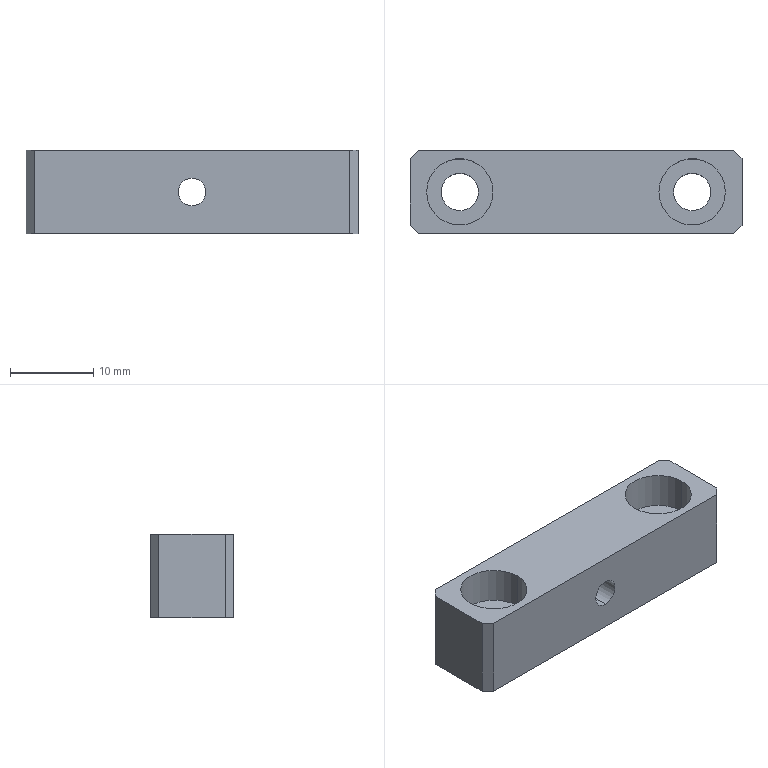Part | STEP file | 11-FG-B08511 | 1 solid | 22 faces | box 40 x 10 x 10 mm | volume 3274 mm3 | plane 12 | cylinder 10 | commonest cylinder face diameters 4.5 x4 8 x4 3.3 x2
STEP:
#1=CARTESIAN_POINT('',(0.,5.,6.65));
#2=VERTEX_POINT('',#1);
#3=CARTESIAN_POINT('',(0.,5.,3.35));
#4=VERTEX_POINT('',#3);
#5=CARTESIAN_POINT('',(0.,5.,5.));
#6=DIRECTION('',(0.,-1.,0.));
#7=DIRECTION('',(0.,0.,-1.));
#8=AXIS2_PLACEMENT_3D('',#5,#6,#7);
#9=CIRCLE('',#8,1.65);
#10=EDGE_CURVE('',#2,#4,#9,.T.);
#11=ORIENTED_EDGE('',*,*,#10,.F.);
#12=CARTESIAN_POINT('',(0.,-5.,6.65));
#13=VERTEX_POINT('',#12);
#14=CARTESIAN_POINT('',(0.,-5.,6.65));
#15=DIRECTION('',(0.,-1.,0.));
#16=VECTOR('',#15,1000.);
#17=LINE('',#14,#16);
#18=EDGE_CURVE('',#2,#13,#17,.T.);
#19=ORIENTED_EDGE('',*,*,#18,.T.);
#20=CARTESIAN_POINT('',(0.,-5.,3.35));
#21=VERTEX_POINT('',#20);
#22=CARTESIAN_POINT('',(0.,-5.,5.));
#23=DIRECTION('',(0.,-1.,0.));
#24=DIRECTION('',(0.,0.,-1.));
#25=AXIS2_PLACEMENT_3D('',#22,#23,#24);
#26=CIRCLE('',#25,1.65);
#27=EDGE_CURVE('',#13,#21,#26,.T.);
#28=ORIENTED_EDGE('',*,*,#27,.T.);
#29=CARTESIAN_POINT('',(0.,-5.,3.35));
#30=DIRECTION('',(0.,-1.,0.));
#31=VECTOR('',#30,1000.);
#32=LINE('',#29,#31);
#33=EDGE_CURVE('',#4,#21,#32,.T.);
#34=ORIENTED_EDGE('',*,*,#33,.F.);
#35=EDGE_LOOP('',(#11,#19,#28,#34));
#36=FACE_OUTER_BOUND('',#35,.T.);
#37=CARTESIAN_POINT('',(0.,-5.,5.));
#38=DIRECTION('',(0.,-1.,0.));
#39=DIRECTION('',(0.,0.,-1.));
#40=AXIS2_PLACEMENT_3D('',#37,#38,#39);
#41=CYLINDRICAL_SURFACE('',#40,1.65);
#42=ADVANCED_FACE('',(#36),#41,.F.);
#43=CARTESIAN_POINT('',(-18.,0.,5.6));
#44=VERTEX_POINT('',#43);
#45=CARTESIAN_POINT('',(-10.,0.,5.6));
#46=VERTEX_POINT('',#45);
#47=CARTESIAN_POINT('',(-14.,0.,5.6));
#48=DIRECTION('',(0.,0.,1.));
#49=DIRECTION('',(1.,0.,0.));
#50=AXIS2_PLACEMENT_3D('',#47,#48,#49);
#51=CIRCLE('',#50,4.);
#52=EDGE_CURVE('',#44,#46,#51,.T.);
#53=ORIENTED_EDGE('',*,*,#52,.F.);
#54=CARTESIAN_POINT('',(-18.,0.,10.));
#55=VERTEX_POINT('',#54);
#56=CARTESIAN_POINT('',(-18.,0.,10.));
#57=DIRECTION('',(0.,0.,1.));
#58=VECTOR('',#57,1000.);
#59=LINE('',#56,#58);
#60=EDGE_CURVE('',#44,#55,#59,.T.);
#61=ORIENTED_EDGE('',*,*,#60,.T.);
#62=CARTESIAN_POINT('',(-10.,0.,10.));
#63=VERTEX_POINT('',#62);
#64=CARTESIAN_POINT('',(-14.,0.,10.));
#65=DIRECTION('',(0.,0.,1.));
#66=DIRECTION('',(1.,0.,0.));
#67=AXIS2_PLACEMENT_3D('',#64,#65,#66);
#68=CIRCLE('',#67,4.);
#69=EDGE_CURVE('',#55,#63,#68,.T.);
#70=ORIENTED_EDGE('',*,*,#69,.T.);
#71=CARTESIAN_POINT('',(-10.,0.,10.));
#72=DIRECTION('',(0.,0.,1.));
#73=VECTOR('',#72,1000.);
#74=LINE('',#71,#73);
#75=EDGE_CURVE('',#46,#63,#74,.T.);
#76=ORIENTED_EDGE('',*,*,#75,.F.);
#77=EDGE_LOOP('',(#53,#61,#70,#76));
#78=FACE_OUTER_BOUND('',#77,.T.);
#79=CARTESIAN_POINT('',(-14.,0.,10.));
#80=DIRECTION('',(0.,0.,1.));
#81=DIRECTION('',(1.,0.,0.));
#82=AXIS2_PLACEMENT_3D('',#79,#80,#81);
#83=CYLINDRICAL_SURFACE('',#82,4.);
#84=ADVANCED_FACE('',(#78),#83,.F.);
#85=CARTESIAN_POINT('',(-11.75,0.,0.));
#86=VERTEX_POINT('',#85);
#87=CARTESIAN_POINT('',(-16.25,0.,0.));
#88=VERTEX_POINT('',#87);
#89=CARTESIAN_POINT('',(-14.,0.,0.));
#90=DIRECTION('',(0.,0.,-1.));
#91=DIRECTION('',(-1.,0.,0.));
#92=AXIS2_PLACEMENT_3D('',#89,#90,#91);
#93=CIRCLE('',#92,2.25);
#94=EDGE_CURVE('',#86,#88,#93,.T.);
#95=ORIENTED_EDGE('',*,*,#94,.T.);
#96=CARTESIAN_POINT('',(-16.25,0.,5.6));
#97=VERTEX_POINT('',#96);
#98=CARTESIAN_POINT('',(-16.25,0.,10.));
#99=DIRECTION('',(0.,0.,1.));
#100=VECTOR('',#99,1000.);
#101=LINE('',#98,#100);
#102=EDGE_CURVE('',#88,#97,#101,.T.);
#103=ORIENTED_EDGE('',*,*,#102,.T.);
#104=CARTESIAN_POINT('',(-11.75,0.,5.6));
#105=VERTEX_POINT('',#104);
#106=CARTESIAN_POINT('',(-14.,0.,5.6));
#107=DIRECTION('',(0.,0.,1.));
#108=DIRECTION('',(1.,0.,0.));
#109=AXIS2_PLACEMENT_3D('',#106,#107,#108);
#110=CIRCLE('',#109,2.25);
#111=EDGE_CURVE('',#97,#105,#110,.T.);
#112=ORIENTED_EDGE('',*,*,#111,.T.);
#113=CARTESIAN_POINT('',(-11.75,0.,10.));
#114=DIRECTION('',(0.,0.,1.));
#115=VECTOR('',#114,1000.);
#116=LINE('',#113,#115);
#117=EDGE_CURVE('',#86,#105,#116,.T.);
#118=ORIENTED_EDGE('',*,*,#117,.F.);
#119=EDGE_LOOP('',(#95,#103,#112,#118));
#120=FACE_OUTER_BOUND('',#119,.T.);
#121=CARTESIAN_POINT('',(-14.,0.,10.));
#122=DIRECTION('',(0.,0.,1.));
#123=DIRECTION('',(1.,0.,0.));
#124=AXIS2_PLACEMENT_3D('',#121,#122,#123);
#125=CYLINDRICAL_SURFACE('',#124,2.25);
#126=ADVANCED_FACE('',(#120),#125,.F.);
#127=CARTESIAN_POINT('',(10.,0.,5.6));
#128=VERTEX_POINT('',#127);
#129=CARTESIAN_POINT('',(18.,0.,5.6));
#130=VERTEX_POINT('',#129);
#131=CARTESIAN_POINT('',(14.,0.,5.6));
#132=DIRECTION('',(0.,0.,1.));
#133=DIRECTION('',(1.,0.,0.));
#134=AXIS2_PLACEMENT_3D('',#131,#132,#133);
#135=CIRCLE('',#134,4.);
#136=EDGE_CURVE('',#128,#130,#135,.T.);
#137=ORIENTED_EDGE('',*,*,#136,.F.);
#138=CARTESIAN_POINT('',(10.,0.,10.));
#139=VERTEX_POINT('',#138);
#140=CARTESIAN_POINT('',(10.,0.,10.));
#141=DIRECTION('',(0.,0.,1.));
#142=VECTOR('',#141,1000.);
#143=LINE('',#140,#142);
#144=EDGE_CURVE('',#128,#139,#143,.T.);
#145=ORIENTED_EDGE('',*,*,#144,.T.);
#146=CARTESIAN_POINT('',(18.,0.,10.));
#147=VERTEX_POINT('',#146);
#148=CARTESIAN_POINT('',(14.,0.,10.));
#149=DIRECTION('',(0.,0.,1.));
#150=DIRECTION('',(1.,0.,0.));
#151=AXIS2_PLACEMENT_3D('',#148,#149,#150);
#152=CIRCLE('',#151,4.);
#153=EDGE_CURVE('',#139,#147,#152,.T.);
#154=ORIENTED_EDGE('',*,*,#153,.T.);
#155=CARTESIAN_POINT('',(18.,0.,10.));
#156=DIRECTION('',(0.,0.,1.));
#157=VECTOR('',#156,1000.);
#158=LINE('',#155,#157);
#159=EDGE_CURVE('',#130,#147,#158,.T.);
#160=ORIENTED_EDGE('',*,*,#159,.F.);
#161=EDGE_LOOP('',(#137,#145,#154,#160));
#162=FACE_OUTER_BOUND('',#161,.T.);
#163=CARTESIAN_POINT('',(14.,0.,10.));
#164=DIRECTION('',(0.,0.,1.));
#165=DIRECTION('',(1.,0.,0.));
#166=AXIS2_PLACEMENT_3D('',#163,#164,#165);
#167=CYLINDRICAL_SURFACE('',#166,4.);
#168=ADVANCED_FACE('',(#162),#167,.F.);
#169=CARTESIAN_POINT('',(16.25,0.,0.));
#170=VERTEX_POINT('',#169);
#171=CARTESIAN_POINT('',(11.75,0.,0.));
#172=VERTEX_POINT('',#171);
#173=CARTESIAN_POINT('',(14.,0.,0.));
#174=DIRECTION('',(0.,0.,-1.));
#175=DIRECTION('',(-1.,0.,0.));
#176=AXIS2_PLACEMENT_3D('',#173,#174,#175);
#177=CIRCLE('',#176,2.25);
#178=EDGE_CURVE('',#170,#172,#177,.T.);
#179=ORIENTED_EDGE('',*,*,#178,.T.);
#180=CARTESIAN_POINT('',(11.75,0.,5.6));
#181=VERTEX_POINT('',#180);
#182=CARTESIAN_POINT('',(11.75,0.,10.));
#183=DIRECTION('',(0.,0.,1.));
#184=VECTOR('',#183,1000.);
#185=LINE('',#182,#184);
#186=EDGE_CURVE('',#172,#181,#185,.T.);
#187=ORIENTED_EDGE('',*,*,#186,.T.);
#188=CARTESIAN_POINT('',(16.25,0.,5.6));
#189=VERTEX_POINT('',#188);
#190=CARTESIAN_POINT('',(14.,0.,5.6));
#191=DIRECTION('',(0.,0.,1.));
#192=DIRECTION('',(1.,0.,0.));
#193=AXIS2_PLACEMENT_3D('',#190,#191,#192);
#194=CIRCLE('',#193,2.25);
#195=EDGE_CURVE('',#181,#189,#194,.T.);
#196=ORIENTED_EDGE('',*,*,#195,.T.);
#197=CARTESIAN_POINT('',(16.25,0.,10.));
#198=DIRECTION('',(0.,0.,1.));
#199=VECTOR('',#198,1000.);
#200=LINE('',#197,#199);
#201=EDGE_CURVE('',#170,#189,#200,.T.);
#202=ORIENTED_EDGE('',*,*,#201,.F.);
#203=EDGE_LOOP('',(#179,#187,#196,#202));
#204=FACE_OUTER_BOUND('',#203,.T.);
#205=CARTESIAN_POINT('',(14.,0.,10.));
#206=DIRECTION('',(0.,0.,1.));
#207=DIRECTION('',(1.,0.,0.));
#208=AXIS2_PLACEMENT_3D('',#205,#206,#207);
#209=CYLINDRICAL_SURFACE('',#208,2.25);
#210=ADVANCED_FACE('',(#204),#209,.F.);
#211=CARTESIAN_POINT('',(20.,-4.,0.));
#212=VERTEX_POINT('',#211);
#213=CARTESIAN_POINT('',(20.,4.,0.));
#214=VERTEX_POINT('',#213);
#215=CARTESIAN_POINT('',(20.,-5.,0.));
#216=DIRECTION('',(0.,1.,0.));
#217=VECTOR('',#216,1000.);
#218=LINE('',#215,#217);
#219=EDGE_CURVE('',#212,#214,#218,.T.);
#220=ORIENTED_EDGE('',*,*,#219,.T.);
#221=CARTESIAN_POINT('',(20.,4.,10.));
#222=VERTEX_POINT('',#221);
#223=CARTESIAN_POINT('',(20.,4.,10.));
#224=DIRECTION('',(0.,0.,1.));
#225=VECTOR('',#224,1000.);
#226=LINE('',#223,#225);
#227=EDGE_CURVE('',#214,#222,#226,.T.);
#228=ORIENTED_EDGE('',*,*,#227,.T.);
#229=CARTESIAN_POINT('',(20.,-4.,10.));
#230=VERTEX_POINT('',#229);
#231=CARTESIAN_POINT('',(20.,-5.,10.));
#232=DIRECTION('',(0.,1.,0.));
#233=VECTOR('',#232,1000.);
#234=LINE('',#231,#233);
#235=EDGE_CURVE('',#230,#222,#234,.T.);
#236=ORIENTED_EDGE('',*,*,#235,.F.);
#237=CARTESIAN_POINT('',(20.,-4.,10.));
#238=DIRECTION('',(0.,0.,-1.));
#239=VECTOR('',#238,1000.);
#240=LINE('',#237,#239);
#241=EDGE_CURVE('',#230,#212,#240,.T.);
#242=ORIENTED_EDGE('',*,*,#241,.T.);
#243=EDGE_LOOP('',(#220,#228,#236,#242));
#244=FACE_OUTER_BOUND('',#243,.T.);
#245=CARTESIAN_POINT('',(20.,-5.,10.));
#246=DIRECTION('',(-1.,0.,0.));
#247=DIRECTION('',(0.,0.,1.));
#248=AXIS2_PLACEMENT_3D('',#245,#246,#247);
#249=PLANE('',#248);
#250=ADVANCED_FACE('',(#244),#249,.F.);
#251=CARTESIAN_POINT('',(0.,5.,5.));
#252=DIRECTION('',(0.,-1.,0.));
#253=DIRECTION('',(0.,0.,-1.));
#254=AXIS2_PLACEMENT_3D('',#251,#252,#253);
#255=CIRCLE('',#254,1.65);
#256=EDGE_CURVE('',#4,#2,#255,.T.);
#257=ORIENTED_EDGE('',*,*,#256,.T.);
#258=ORIENTED_EDGE('',*,*,#10,.T.);
#259=EDGE_LOOP('',(#257,#258));
#260=FACE_BOUND('',#259,.T.);
#261=CARTESIAN_POINT('',(19.,5.,10.));
#262=VERTEX_POINT('',#261);
#263=CARTESIAN_POINT('',(-19.,5.,10.));
#264=VERTEX_POINT('',#263);
#265=CARTESIAN_POINT('',(-20.,5.,10.));
#266=DIRECTION('',(-1.,0.,0.));
#267=VECTOR('',#266,1000.);
#268=LINE('',#265,#267);
#269=EDGE_CURVE('',#262,#264,#268,.T.);
#270=ORIENTED_EDGE('',*,*,#269,.F.);
#271=CARTESIAN_POINT('',(19.,5.,0.));
#272=VERTEX_POINT('',#271);
#273=CARTESIAN_POINT('',(19.,5.,10.));
#274=DIRECTION('',(0.,0.,-1.));
#275=VECTOR('',#274,1000.);
#276=LINE('',#273,#275);
#277=EDGE_CURVE('',#262,#272,#276,.T.);
#278=ORIENTED_EDGE('',*,*,#277,.T.);
#279=CARTESIAN_POINT('',(-19.,5.,0.));
#280=VERTEX_POINT('',#279);
#281=CARTESIAN_POINT('',(-20.,5.,0.));
#282=DIRECTION('',(-1.,0.,0.));
#283=VECTOR('',#282,1000.);
#284=LINE('',#281,#283);
#285=EDGE_CURVE('',#272,#280,#284,.T.);
#286=ORIENTED_EDGE('',*,*,#285,.T.);
#287=CARTESIAN_POINT('',(-19.,5.,10.));
#288=DIRECTION('',(0.,0.,1.));
#289=VECTOR('',#288,1000.);
#290=LINE('',#287,#289);
#291=EDGE_CURVE('',#280,#264,#290,.T.);
#292=ORIENTED_EDGE('',*,*,#291,.T.);
#293=EDGE_LOOP('',(#270,#278,#286,#292));
#294=FACE_OUTER_BOUND('',#293,.T.);
#295=CARTESIAN_POINT('',(-20.,5.,10.));
#296=DIRECTION('',(0.,-1.,0.));
#297=DIRECTION('',(0.,0.,-1.));
#298=AXIS2_PLACEMENT_3D('',#295,#296,#297);
#299=PLANE('',#298);
#300=ADVANCED_FACE('',(#260,#294),#299,.F.);
#301=CARTESIAN_POINT('',(-20.,4.,0.));
#302=VERTEX_POINT('',#301);
#303=CARTESIAN_POINT('',(-20.,-4.,0.));
#304=VERTEX_POINT('',#303);
#305=CARTESIAN_POINT('',(-20.,-5.,0.));
#306=DIRECTION('',(0.,-1.,0.));
#307=VECTOR('',#306,1000.);
#308=LINE('',#305,#307);
#309=EDGE_CURVE('',#302,#304,#308,.T.);
#310=ORIENTED_EDGE('',*,*,#309,.T.);
#311=CARTESIAN_POINT('',(-20.,-4.,10.));
#312=VERTEX_POINT('',#311);
#313=CARTESIAN_POINT('',(-20.,-4.,10.));
#314=DIRECTION('',(0.,0.,1.));
#315=VECTOR('',#314,1000.);
#316=LINE('',#313,#315);
#317=EDGE_CURVE('',#304,#312,#316,.T.);
#318=ORIENTED_EDGE('',*,*,#317,.T.);
#319=CARTESIAN_POINT('',(-20.,4.,10.));
#320=VERTEX_POINT('',#319);
#321=CARTESIAN_POINT('',(-20.,-5.,10.));
#322=DIRECTION('',(0.,-1.,0.));
#323=VECTOR('',#322,1000.);
#324=LINE('',#321,#323);
#325=EDGE_CURVE('',#320,#312,#324,.T.);
#326=ORIENTED_EDGE('',*,*,#325,.F.);
#327=CARTESIAN_POINT('',(-20.,4.,10.));
#328=DIRECTION('',(0.,0.,-1.));
#329=VECTOR('',#328,1000.);
#330=LINE('',#327,#329);
#331=EDGE_CURVE('',#320,#302,#330,.T.);
#332=ORIENTED_EDGE('',*,*,#331,.T.);
#333=EDGE_LOOP('',(#310,#318,#326,#332));
#334=FACE_OUTER_BOUND('',#333,.T.);
#335=CARTESIAN_POINT('',(-20.,-5.,10.));
#336=DIRECTION('',(1.,0.,0.));
#337=DIRECTION('',(0.,0.,-1.));
#338=AXIS2_PLACEMENT_3D('',#335,#336,#337);
#339=PLANE('',#338);
#340=ADVANCED_FACE('',(#334),#339,.F.);
#341=CARTESIAN_POINT('',(0.,-5.,5.));
#342=DIRECTION('',(0.,-1.,0.));
#343=DIRECTION('',(0.,0.,-1.));
#344=AXIS2_PLACEMENT_3D('',#341,#342,#343);
#345=CIRCLE('',#344,1.65);
#346=EDGE_CURVE('',#21,#13,#345,.T.);
#347=ORIENTED_EDGE('',*,*,#346,.F.);
#348=ORIENTED_EDGE('',*,*,#27,.F.);
#349=EDGE_LOOP('',(#347,#348));
#350=FACE_BOUND('',#349,.T.);
#351=CARTESIAN_POINT('',(-19.,-5.,0.));
#352=VERTEX_POINT('',#351);
#353=CARTESIAN_POINT('',(19.,-5.,0.));
#354=VERTEX_POINT('',#353);
#355=CARTESIAN_POINT('',(-20.,-5.,0.));
#356=DIRECTION('',(1.,0.,0.));
#357=VECTOR('',#356,1000.);
#358=LINE('',#355,#357);
#359=EDGE_CURVE('',#352,#354,#358,.T.);
#360=ORIENTED_EDGE('',*,*,#359,.T.);
#361=CARTESIAN_POINT('',(19.,-5.,10.));
#362=VERTEX_POINT('',#361);
#363=CARTESIAN_POINT('',(19.,-5.,10.));
#364=DIRECTION('',(0.,0.,1.));
#365=VECTOR('',#364,1000.);
#366=LINE('',#363,#365);
#367=EDGE_CURVE('',#354,#362,#366,.T.);
#368=ORIENTED_EDGE('',*,*,#367,.T.);
#369=CARTESIAN_POINT('',(-19.,-5.,10.));
#370=VERTEX_POINT('',#369);
#371=CARTESIAN_POINT('',(-20.,-5.,10.));
#372=DIRECTION('',(1.,0.,0.));
#373=VECTOR('',#372,1000.);
#374=LINE('',#371,#373);
#375=EDGE_CURVE('',#370,#362,#374,.T.);
#376=ORIENTED_EDGE('',*,*,#375,.F.);
#377=CARTESIAN_POINT('',(-19.,-5.,10.));
#378=DIRECTION('',(0.,0.,-1.));
#379=VECTOR('',#378,1000.);
#380=LINE('',#377,#379);
#381=EDGE_CURVE('',#370,#352,#380,.T.);
#382=ORIENTED_EDGE('',*,*,#381,.T.);
#383=EDGE_LOOP('',(#360,#368,#376,#382));
#384=FACE_OUTER_BOUND('',#383,.T.);
#385=CARTESIAN_POINT('',(-20.,-5.,10.));
#386=DIRECTION('',(0.,1.,0.));
#387=DIRECTION('',(0.,0.,1.));
#388=AXIS2_PLACEMENT_3D('',#385,#386,#387);
#389=PLANE('',#388);
#390=ADVANCED_FACE('',(#350,#384),#389,.F.);
#391=CARTESIAN_POINT('',(-14.,0.,10.));
#392=DIRECTION('',(0.,0.,1.));
#393=DIRECTION('',(1.,0.,0.));
#394=AXIS2_PLACEMENT_3D('',#391,#392,#393);
#395=CIRCLE('',#394,4.);
#396=EDGE_CURVE('',#63,#55,#395,.T.);
#397=ORIENTED_EDGE('',*,*,#396,.F.);
#398=ORIENTED_EDGE('',*,*,#69,.F.);
#399=EDGE_LOOP('',(#397,#398));
#400=FACE_BOUND('',#399,.T.);
#401=CARTESIAN_POINT('',(14.,0.,10.));
#402=DIRECTION('',(0.,0.,1.));
#403=DIRECTION('',(1.,0.,0.));
#404=AXIS2_PLACEMENT_3D('',#401,#402,#403);
#405=CIRCLE('',#404,4.);
#406=EDGE_CURVE('',#147,#139,#405,.T.);
#407=ORIENTED_EDGE('',*,*,#406,.F.);
#408=ORIENTED_EDGE('',*,*,#153,.F.);
#409=EDGE_LOOP('',(#407,#408));
#410=FACE_BOUND('',#409,.T.);
#411=ORIENTED_EDGE('',*,*,#235,.T.);
#412=CARTESIAN_POINT('',(19.,5.,10.));
#413=DIRECTION('',(-0.7071,0.7071,0.));
#414=VECTOR('',#413,1000.);
#415=LINE('',#412,#414);
#416=EDGE_CURVE('',#222,#262,#415,.T.);
#417=ORIENTED_EDGE('',*,*,#416,.T.);
#418=ORIENTED_EDGE('',*,*,#269,.T.);
#419=CARTESIAN_POINT('',(-20.,4.,10.));
#420=DIRECTION('',(-0.7071,-0.7071,0.));
#421=VECTOR('',#420,1000.);
#422=LINE('',#419,#421);
#423=EDGE_CURVE('',#264,#320,#422,.T.);
#424=ORIENTED_EDGE('',*,*,#423,.T.);
#425=ORIENTED_EDGE('',*,*,#325,.T.);
#426=CARTESIAN_POINT('',(-19.,-5.,10.));
#427=DIRECTION('',(0.7071,-0.7071,0.));
#428=VECTOR('',#427,1000.);
#429=LINE('',#426,#428);
#430=EDGE_CURVE('',#312,#370,#429,.T.);
#431=ORIENTED_EDGE('',*,*,#430,.T.);
#432=ORIENTED_EDGE('',*,*,#375,.T.);
#433=CARTESIAN_POINT('',(20.,-4.,10.));
#434=DIRECTION('',(0.7071,0.7071,0.));
#435=VECTOR('',#434,1000.);
#436=LINE('',#433,#435);
#437=EDGE_CURVE('',#362,#230,#436,.T.);
#438=ORIENTED_EDGE('',*,*,#437,.T.);
#439=EDGE_LOOP('',(#411,#417,#418,#424,#425,#431,#432,#438));
#440=FACE_OUTER_BOUND('',#439,.T.);
#441=CARTESIAN_POINT('',(20.,5.,10.));
#442=DIRECTION('',(0.,0.,-1.));
#443=DIRECTION('',(-1.,0.,0.));
#444=AXIS2_PLACEMENT_3D('',#441,#442,#443);
#445=PLANE('',#444);
#446=ADVANCED_FACE('',(#400,#410,#440),#445,.F.);
#447=ORIENTED_EDGE('',*,*,#94,.F.);
#448=CARTESIAN_POINT('',(-14.,0.,0.));
#449=DIRECTION('',(0.,0.,-1.));
#450=DIRECTION('',(-1.,0.,0.));
#451=AXIS2_PLACEMENT_3D('',#448,#449,#450);
#452=CIRCLE('',#451,2.25);
#453=EDGE_CURVE('',#88,#86,#452,.T.);
#454=ORIENTED_EDGE('',*,*,#453,.F.);
#455=EDGE_LOOP('',(#447,#454));
#456=FACE_BOUND('',#455,.T.);
#457=ORIENTED_EDGE('',*,*,#178,.F.);
#458=CARTESIAN_POINT('',(14.,0.,0.));
#459=DIRECTION('',(0.,0.,-1.));
#460=DIRECTION('',(-1.,0.,0.));
#461=AXIS2_PLACEMENT_3D('',#458,#459,#460);
#462=CIRCLE('',#461,2.25);
#463=EDGE_CURVE('',#172,#170,#462,.T.);
#464=ORIENTED_EDGE('',*,*,#463,.F.);
#465=EDGE_LOOP('',(#457,#464));
#466=FACE_BOUND('',#465,.T.);
#467=ORIENTED_EDGE('',*,*,#285,.F.);
#468=CARTESIAN_POINT('',(19.5,4.5,0.));
#469=DIRECTION('',(0.7071,-0.7071,0.));
#470=VECTOR('',#469,1000.);
#471=LINE('',#468,#470);
#472=EDGE_CURVE('',#272,#214,#471,.T.);
#473=ORIENTED_EDGE('',*,*,#472,.T.);
#474=ORIENTED_EDGE('',*,*,#219,.F.);
#475=CARTESIAN_POINT('',(24.5,0.5,0.));
#476=DIRECTION('',(-0.7071,-0.7071,0.));
#477=VECTOR('',#476,1000.);
#478=LINE('',#475,#477);
#479=EDGE_CURVE('',#212,#354,#478,.T.);
#480=ORIENTED_EDGE('',*,*,#479,.T.);
#481=ORIENTED_EDGE('',*,*,#359,.F.);
#482=CARTESIAN_POINT('',(-4.5,-19.5,0.));
#483=DIRECTION('',(-0.7071,0.7071,0.));
#484=VECTOR('',#483,1000.);
#485=LINE('',#482,#484);
#486=EDGE_CURVE('',#352,#304,#485,.T.);
#487=ORIENTED_EDGE('',*,*,#486,.T.);
#488=ORIENTED_EDGE('',*,*,#309,.F.);
#489=CARTESIAN_POINT('',(0.5,24.5,0.));
#490=DIRECTION('',(0.7071,0.7071,0.));
#491=VECTOR('',#490,1000.);
#492=LINE('',#489,#491);
#493=EDGE_CURVE('',#302,#280,#492,.T.);
#494=ORIENTED_EDGE('',*,*,#493,.T.);
#495=EDGE_LOOP('',(#467,#473,#474,#480,#481,#487,#488,#494));
#496=FACE_OUTER_BOUND('',#495,.T.);
#497=CARTESIAN_POINT('',(20.,5.,0.));
#498=DIRECTION('',(0.,0.,-1.));
#499=DIRECTION('',(-1.,0.,0.));
#500=AXIS2_PLACEMENT_3D('',#497,#498,#499);
#501=PLANE('',#500);
#502=ADVANCED_FACE('',(#456,#466,#496),#501,.T.);
#503=ORIENTED_EDGE('',*,*,#416,.F.);
#504=ORIENTED_EDGE('',*,*,#227,.F.);
#505=ORIENTED_EDGE('',*,*,#472,.F.);
#506=ORIENTED_EDGE('',*,*,#277,.F.);
#507=EDGE_LOOP('',(#503,#504,#505,#506));
#508=FACE_OUTER_BOUND('',#507,.T.);
#509=CARTESIAN_POINT('',(19.,5.,10.));
#510=DIRECTION('',(-0.7071,-0.7071,0.));
#511=DIRECTION('',(0.,0.,-1.));
#512=AXIS2_PLACEMENT_3D('',#509,#510,#511);
#513=PLANE('',#512);
#514=ADVANCED_FACE('',(#508),#513,.F.);
#515=ORIENTED_EDGE('',*,*,#437,.F.);
#516=ORIENTED_EDGE('',*,*,#367,.F.);
#517=ORIENTED_EDGE('',*,*,#479,.F.);
#518=ORIENTED_EDGE('',*,*,#241,.F.);
#519=EDGE_LOOP('',(#515,#516,#517,#518));
#520=FACE_OUTER_BOUND('',#519,.T.);
#521=CARTESIAN_POINT('',(20.,-4.,10.));
#522=DIRECTION('',(-0.7071,0.7071,0.));
#523=DIRECTION('',(0.,0.,-1.));
#524=AXIS2_PLACEMENT_3D('',#521,#522,#523);
#525=PLANE('',#524);
#526=ADVANCED_FACE('',(#520),#525,.F.);
#527=ORIENTED_EDGE('',*,*,#430,.F.);
#528=ORIENTED_EDGE('',*,*,#317,.F.);
#529=ORIENTED_EDGE('',*,*,#486,.F.);
#530=ORIENTED_EDGE('',*,*,#381,.F.);
#531=EDGE_LOOP('',(#527,#528,#529,#530));
#532=FACE_OUTER_BOUND('',#531,.T.);
#533=CARTESIAN_POINT('',(-19.,-5.,10.));
#534=DIRECTION('',(0.7071,0.7071,0.));
#535=DIRECTION('',(0.,0.,-1.));
#536=AXIS2_PLACEMENT_3D('',#533,#534,#535);
#537=PLANE('',#536);
#538=ADVANCED_FACE('',(#532),#537,.F.);
#539=ORIENTED_EDGE('',*,*,#423,.F.);
#540=ORIENTED_EDGE('',*,*,#291,.F.);
#541=ORIENTED_EDGE('',*,*,#493,.F.);
#542=ORIENTED_EDGE('',*,*,#331,.F.);
#543=EDGE_LOOP('',(#539,#540,#541,#542));
#544=FACE_OUTER_BOUND('',#543,.T.);
#545=CARTESIAN_POINT('',(-20.,4.,10.));
#546=DIRECTION('',(0.7071,-0.7071,0.));
#547=DIRECTION('',(0.,0.,-1.));
#548=AXIS2_PLACEMENT_3D('',#545,#546,#547);
#549=PLANE('',#548);
#550=ADVANCED_FACE('',(#544),#549,.F.);
#551=ORIENTED_EDGE('',*,*,#186,.F.);
#552=ORIENTED_EDGE('',*,*,#463,.T.);
#553=ORIENTED_EDGE('',*,*,#201,.T.);
#554=CARTESIAN_POINT('',(14.,0.,5.6));
#555=DIRECTION('',(0.,0.,1.));
#556=DIRECTION('',(1.,0.,0.));
#557=AXIS2_PLACEMENT_3D('',#554,#555,#556);
#558=CIRCLE('',#557,2.25);
#559=EDGE_CURVE('',#189,#181,#558,.T.);
#560=ORIENTED_EDGE('',*,*,#559,.T.);
#561=EDGE_LOOP('',(#551,#552,#553,#560));
#562=FACE_OUTER_BOUND('',#561,.T.);
#563=CARTESIAN_POINT('',(14.,0.,10.));
#564=DIRECTION('',(0.,0.,1.));
#565=DIRECTION('',(1.,0.,0.));
#566=AXIS2_PLACEMENT_3D('',#563,#564,#565);
#567=CYLINDRICAL_SURFACE('',#566,2.25);
#568=ADVANCED_FACE('',(#562),#567,.F.);
#569=ORIENTED_EDGE('',*,*,#559,.F.);
#570=ORIENTED_EDGE('',*,*,#195,.F.);
#571=EDGE_LOOP('',(#569,#570));
#572=FACE_BOUND('',#571,.T.);
#573=CARTESIAN_POINT('',(14.,0.,5.6));
#574=DIRECTION('',(0.,0.,1.));
#575=DIRECTION('',(1.,0.,0.));
#576=AXIS2_PLACEMENT_3D('',#573,#574,#575);
#577=CIRCLE('',#576,4.);
#578=EDGE_CURVE('',#130,#128,#577,.T.);
#579=ORIENTED_EDGE('',*,*,#578,.T.);
#580=ORIENTED_EDGE('',*,*,#136,.T.);
#581=EDGE_LOOP('',(#579,#580));
#582=FACE_OUTER_BOUND('',#581,.T.);
#583=CARTESIAN_POINT('',(16.25,0.,5.6));
#584=DIRECTION('',(0.,0.,-1.));
#585=DIRECTION('',(-1.,0.,0.));
#586=AXIS2_PLACEMENT_3D('',#583,#584,#585);
#587=PLANE('',#586);
#588=ADVANCED_FACE('',(#572,#582),#587,.F.);
#589=ORIENTED_EDGE('',*,*,#144,.F.);
#590=ORIENTED_EDGE('',*,*,#578,.F.);
#591=ORIENTED_EDGE('',*,*,#159,.T.);
#592=ORIENTED_EDGE('',*,*,#406,.T.);
#593=EDGE_LOOP('',(#589,#590,#591,#592));
#594=FACE_OUTER_BOUND('',#593,.T.);
#595=CARTESIAN_POINT('',(14.,0.,10.));
#596=DIRECTION('',(0.,0.,1.));
#597=DIRECTION('',(1.,0.,0.));
#598=AXIS2_PLACEMENT_3D('',#595,#596,#597);
#599=CYLINDRICAL_SURFACE('',#598,4.);
#600=ADVANCED_FACE('',(#594),#599,.F.);
#601=ORIENTED_EDGE('',*,*,#102,.F.);
#602=ORIENTED_EDGE('',*,*,#453,.T.);
#603=ORIENTED_EDGE('',*,*,#117,.T.);
#604=CARTESIAN_POINT('',(-14.,0.,5.6));
#605=DIRECTION('',(0.,0.,1.));
#606=DIRECTION('',(1.,0.,0.));
#607=AXIS2_PLACEMENT_3D('',#604,#605,#606);
#608=CIRCLE('',#607,2.25);
#609=EDGE_CURVE('',#105,#97,#608,.T.);
#610=ORIENTED_EDGE('',*,*,#609,.T.);
#611=EDGE_LOOP('',(#601,#602,#603,#610));
#612=FACE_OUTER_BOUND('',#611,.T.);
#613=CARTESIAN_POINT('',(-14.,0.,10.));
#614=DIRECTION('',(0.,0.,1.));
#615=DIRECTION('',(1.,0.,0.));
#616=AXIS2_PLACEMENT_3D('',#613,#614,#615);
#617=CYLINDRICAL_SURFACE('',#616,2.25);
#618=ADVANCED_FACE('',(#612),#617,.F.);
#619=ORIENTED_EDGE('',*,*,#609,.F.);
#620=ORIENTED_EDGE('',*,*,#111,.F.);
#621=EDGE_LOOP('',(#619,#620));
#622=FACE_BOUND('',#621,.T.);
#623=CARTESIAN_POINT('',(-14.,0.,5.6));
#624=DIRECTION('',(0.,0.,1.));
#625=DIRECTION('',(1.,0.,0.));
#626=AXIS2_PLACEMENT_3D('',#623,#624,#625);
#627=CIRCLE('',#626,4.);
#628=EDGE_CURVE('',#46,#44,#627,.T.);
#629=ORIENTED_EDGE('',*,*,#628,.T.);
#630=ORIENTED_EDGE('',*,*,#52,.T.);
#631=EDGE_LOOP('',(#629,#630));
#632=FACE_OUTER_BOUND('',#631,.T.);
#633=CARTESIAN_POINT('',(-11.75,0.,5.6));
#634=DIRECTION('',(0.,0.,-1.));
#635=DIRECTION('',(-1.,0.,0.));
#636=AXIS2_PLACEMENT_3D('',#633,#634,#635);
#637=PLANE('',#636);
#638=ADVANCED_FACE('',(#622,#632),#637,.F.);
#639=ORIENTED_EDGE('',*,*,#60,.F.);
#640=ORIENTED_EDGE('',*,*,#628,.F.);
#641=ORIENTED_EDGE('',*,*,#75,.T.);
#642=ORIENTED_EDGE('',*,*,#396,.T.);
#643=EDGE_LOOP('',(#639,#640,#641,#642));
#644=FACE_OUTER_BOUND('',#643,.T.);
#645=CARTESIAN_POINT('',(-14.,0.,10.));
#646=DIRECTION('',(0.,0.,1.));
#647=DIRECTION('',(1.,0.,0.));
#648=AXIS2_PLACEMENT_3D('',#645,#646,#647);
#649=CYLINDRICAL_SURFACE('',#648,4.);
#650=ADVANCED_FACE('',(#644),#649,.F.);
#651=ORIENTED_EDGE('',*,*,#18,.F.);
#652=ORIENTED_EDGE('',*,*,#256,.F.);
#653=ORIENTED_EDGE('',*,*,#33,.T.);
#654=ORIENTED_EDGE('',*,*,#346,.T.);
#655=EDGE_LOOP('',(#651,#652,#653,#654));
#656=FACE_OUTER_BOUND('',#655,.T.);
#657=CARTESIAN_POINT('',(0.,-5.,5.));
#658=DIRECTION('',(0.,-1.,0.));
#659=DIRECTION('',(0.,0.,-1.));
#660=AXIS2_PLACEMENT_3D('',#657,#658,#659);
#661=CYLINDRICAL_SURFACE('',#660,1.65);
#662=ADVANCED_FACE('',(#656),#661,.F.);
#663=CLOSED_SHELL('',(#42,#84,#126,#168,#210,#250,#300,#340,#390,#446,#502,#514,#526,#538,#550,#568,#588,#600,#618,#638,#650,#662));
#664=MANIFOLD_SOLID_BREP('',#663);
#665=CARTESIAN_POINT('',(0.,0.,0.));
#666=DIRECTION('',(0.,0.,1.));
#667=DIRECTION('',(1.,0.,0.));
#668=AXIS2_PLACEMENT_3D('',#665,#666,#667);
#669=(LENGTH_UNIT()NAMED_UNIT(*)SI_UNIT(.MILLI.,.METRE.));
#670=UNCERTAINTY_MEASURE_WITH_UNIT(LENGTH_MEASURE(0.00001),#669,'','');
#671=(NAMED_UNIT(*)PLANE_ANGLE_UNIT()SI_UNIT($,.RADIAN.));
#672=(NAMED_UNIT(*)SI_UNIT($,.STERADIAN.)SOLID_ANGLE_UNIT());
#673=(GEOMETRIC_REPRESENTATION_CONTEXT(3)GLOBAL_UNCERTAINTY_ASSIGNED_CONTEXT((#670))GLOBAL_UNIT_ASSIGNED_CONTEXT((#669,#671,#672))REPRESENTATION_CONTEXT('',''));
#674=ADVANCED_BREP_SHAPE_REPRESENTATION('',(#664,#668),#673);